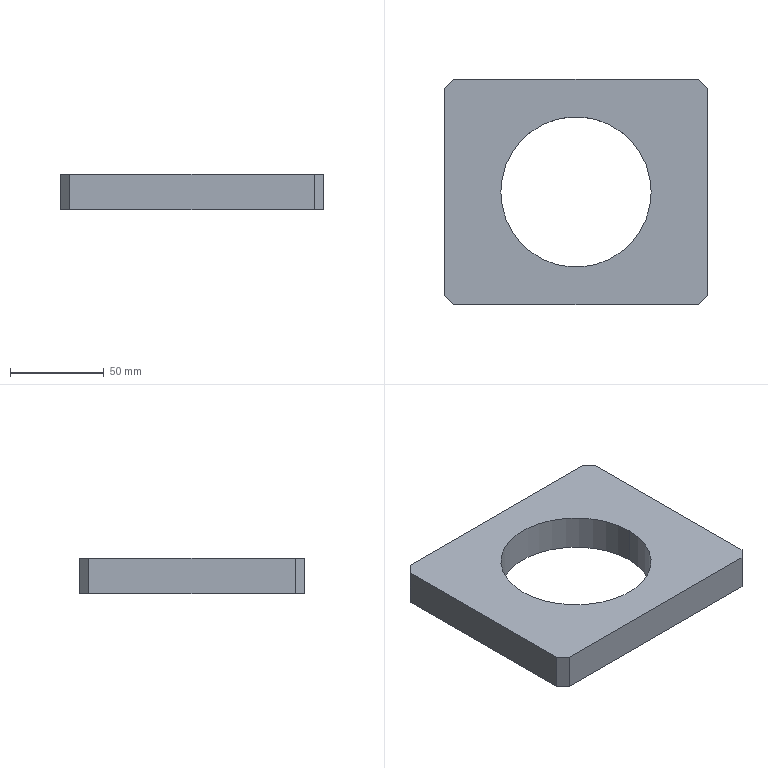Part | STEP file | Backup 2012-3-22-017 | 1 solid | 12 faces | box 140 x 120 x 19 mm | volume 222746 mm3 | plane 10 | cylinder 2 | commonest cylinder face diameters 80 x2
STEP:
#1=CARTESIAN_POINT('',(0.,0.,0.));
#2=DIRECTION('',(0.,0.,1.));
#3=DIRECTION('',(1.,0.,0.));
#4=AXIS2_PLACEMENT_3D('',#1,#2,#3);
#5=CARTESIAN_POINT('',(-40.,0.,19.));
#6=VERTEX_POINT('',#5);
#7=CARTESIAN_POINT('',(-40.,0.,0.));
#8=VERTEX_POINT('',#7);
#9=CARTESIAN_POINT('',(-40.,0.,19.));
#10=DIRECTION('',(0.,0.,-1.));
#11=VECTOR('',#10,1.);
#12=LINE('',#9,#11);
#13=CARTESIAN_POINT('',(0.,0.,19.));
#14=DIRECTION('',(0.,0.,-1.));
#15=DIRECTION('',(-1.,0.,0.));
#16=AXIS2_PLACEMENT_3D('',#13,#14,#15);
#17=CYLINDRICAL_SURFACE('',#16,40.);
#18=CARTESIAN_POINT('',(6.283,0.));
#19=DIRECTION('',(0.,1.));
#20=VECTOR('',#19,1.);
#21=LINE('',#18,#20);
#22=(GEOMETRIC_REPRESENTATION_CONTEXT(2)PARAMETRIC_REPRESENTATION_CONTEXT()REPRESENTATION_CONTEXT('',''));
#23=DEFINITIONAL_REPRESENTATION('',(#21),#22);
#24=PCURVE('',#17,#23);
#25=CARTESIAN_POINT('',(0.,0.,19.));
#26=DIRECTION('',(0.,0.,-1.));
#27=DIRECTION('',(-1.,0.,0.));
#28=AXIS2_PLACEMENT_3D('',#25,#26,#27);
#29=CYLINDRICAL_SURFACE('',#28,40.);
#30=CARTESIAN_POINT('',(0.,0.));
#31=DIRECTION('',(0.,1.));
#32=VECTOR('',#31,1.);
#33=LINE('',#30,#32);
#34=(GEOMETRIC_REPRESENTATION_CONTEXT(2)PARAMETRIC_REPRESENTATION_CONTEXT()REPRESENTATION_CONTEXT('',''));
#35=DEFINITIONAL_REPRESENTATION('',(#33),#34);
#36=PCURVE('',#29,#35);
#37=SURFACE_CURVE('',#12,(#24,#36),.PCURVE_S1.);
#38=EDGE_CURVE('',#6,#8,#37,.T.);
#39=ORIENTED_EDGE('',*,*,#38,.T.);
#40=CARTESIAN_POINT('',(40.,0.,0.));
#41=VERTEX_POINT('',#40);
#42=CARTESIAN_POINT('',(0.,0.,0.));
#43=DIRECTION('',(0.,0.,1.));
#44=DIRECTION('',(1.,0.,0.));
#45=AXIS2_PLACEMENT_3D('',#42,#43,#44);
#46=CIRCLE('',#45,40.);
#47=CARTESIAN_POINT('',(9.425,19.));
#48=DIRECTION('',(-1.,0.));
#49=VECTOR('',#48,1.);
#50=LINE('',#47,#49);
#51=(GEOMETRIC_REPRESENTATION_CONTEXT(2)PARAMETRIC_REPRESENTATION_CONTEXT()REPRESENTATION_CONTEXT('',''));
#52=DEFINITIONAL_REPRESENTATION('',(#50),#51);
#53=PCURVE('',#17,#52);
#54=CARTESIAN_POINT('',(70.,-60.,0.));
#55=DIRECTION('',(0.,0.,1.));
#56=DIRECTION('',(1.,0.,0.));
#57=AXIS2_PLACEMENT_3D('',#54,#55,#56);
#58=PLANE('',#57);
#59=CARTESIAN_POINT('',(-70.,60.));
#60=DIRECTION('',(1.,0.));
#61=AXIS2_PLACEMENT_2D('',#59,#60);
#62=CIRCLE('',#61,40.);
#63=(GEOMETRIC_REPRESENTATION_CONTEXT(2)PARAMETRIC_REPRESENTATION_CONTEXT()REPRESENTATION_CONTEXT('',''));
#64=DEFINITIONAL_REPRESENTATION('',(#62),#63);
#65=PCURVE('',#58,#64);
#66=SURFACE_CURVE('',#46,(#53,#65),.PCURVE_S1.);
#67=EDGE_CURVE('',#8,#41,#66,.T.);
#68=ORIENTED_EDGE('',*,*,#67,.T.);
#69=CARTESIAN_POINT('',(40.,0.,19.));
#70=VERTEX_POINT('',#69);
#71=CARTESIAN_POINT('',(40.,0.,19.));
#72=DIRECTION('',(0.,0.,-1.));
#73=VECTOR('',#72,1.);
#74=LINE('',#71,#73);
#75=CARTESIAN_POINT('',(3.142,0.));
#76=DIRECTION('',(0.,1.));
#77=VECTOR('',#76,1.);
#78=LINE('',#75,#77);
#79=(GEOMETRIC_REPRESENTATION_CONTEXT(2)PARAMETRIC_REPRESENTATION_CONTEXT()REPRESENTATION_CONTEXT('',''));
#80=DEFINITIONAL_REPRESENTATION('',(#78),#79);
#81=PCURVE('',#17,#80);
#82=CARTESIAN_POINT('',(3.142,0.));
#83=DIRECTION('',(0.,1.));
#84=VECTOR('',#83,1.);
#85=LINE('',#82,#84);
#86=(GEOMETRIC_REPRESENTATION_CONTEXT(2)PARAMETRIC_REPRESENTATION_CONTEXT()REPRESENTATION_CONTEXT('',''));
#87=DEFINITIONAL_REPRESENTATION('',(#85),#86);
#88=PCURVE('',#29,#87);
#89=SURFACE_CURVE('',#74,(#81,#88),.PCURVE_S1.);
#90=EDGE_CURVE('',#70,#41,#89,.T.);
#91=ORIENTED_EDGE('',*,*,#90,.F.);
#92=CARTESIAN_POINT('',(0.,0.,19.));
#93=DIRECTION('',(0.,0.,1.));
#94=DIRECTION('',(1.,0.,0.));
#95=AXIS2_PLACEMENT_3D('',#92,#93,#94);
#96=CIRCLE('',#95,40.);
#97=CARTESIAN_POINT('',(9.425,0.));
#98=DIRECTION('',(-1.,0.));
#99=VECTOR('',#98,1.);
#100=LINE('',#97,#99);
#101=(GEOMETRIC_REPRESENTATION_CONTEXT(2)PARAMETRIC_REPRESENTATION_CONTEXT()REPRESENTATION_CONTEXT('',''));
#102=DEFINITIONAL_REPRESENTATION('',(#100),#101);
#103=PCURVE('',#17,#102);
#104=CARTESIAN_POINT('',(70.,-60.,19.));
#105=DIRECTION('',(0.,0.,1.));
#106=DIRECTION('',(1.,0.,0.));
#107=AXIS2_PLACEMENT_3D('',#104,#105,#106);
#108=PLANE('',#107);
#109=CARTESIAN_POINT('',(-70.,60.));
#110=DIRECTION('',(1.,0.));
#111=AXIS2_PLACEMENT_2D('',#109,#110);
#112=CIRCLE('',#111,40.);
#113=(GEOMETRIC_REPRESENTATION_CONTEXT(2)PARAMETRIC_REPRESENTATION_CONTEXT()REPRESENTATION_CONTEXT('',''));
#114=DEFINITIONAL_REPRESENTATION('',(#112),#113);
#115=PCURVE('',#108,#114);
#116=SURFACE_CURVE('',#96,(#103,#115),.PCURVE_S1.);
#117=EDGE_CURVE('',#6,#70,#116,.T.);
#118=ORIENTED_EDGE('',*,*,#117,.F.);
#119=EDGE_LOOP('',(#39,#68,#91,#118));
#120=FACE_BOUND('',#119,.F.);
#121=ADVANCED_FACE('',(#120),#17,.F.);
#122=CARTESIAN_POINT('',(-70.,55.,19.));
#123=VERTEX_POINT('',#122);
#124=CARTESIAN_POINT('',(-70.,-55.,19.));
#125=VERTEX_POINT('',#124);
#126=CARTESIAN_POINT('',(-70.,60.,19.));
#127=DIRECTION('',(0.,-1.,0.));
#128=VECTOR('',#127,1.);
#129=LINE('',#126,#128);
#130=CARTESIAN_POINT('',(-140.,120.));
#131=DIRECTION('',(0.,-1.));
#132=VECTOR('',#131,1.);
#133=LINE('',#130,#132);
#134=(GEOMETRIC_REPRESENTATION_CONTEXT(2)PARAMETRIC_REPRESENTATION_CONTEXT()REPRESENTATION_CONTEXT('',''));
#135=DEFINITIONAL_REPRESENTATION('',(#133),#134);
#136=PCURVE('',#108,#135);
#137=CARTESIAN_POINT('',(-70.,60.,19.));
#138=DIRECTION('',(1.,0.,0.));
#139=DIRECTION('',(0.,0.,-1.));
#140=AXIS2_PLACEMENT_3D('',#137,#138,#139);
#141=PLANE('',#140);
#142=CARTESIAN_POINT('',(0.,0.));
#143=DIRECTION('',(0.,-1.));
#144=VECTOR('',#143,1.);
#145=LINE('',#142,#144);
#146=(GEOMETRIC_REPRESENTATION_CONTEXT(2)PARAMETRIC_REPRESENTATION_CONTEXT()REPRESENTATION_CONTEXT('',''));
#147=DEFINITIONAL_REPRESENTATION('',(#145),#146);
#148=PCURVE('',#141,#147);
#149=SURFACE_CURVE('',#129,(#136,#148),.PCURVE_S1.);
#150=EDGE_CURVE('',#123,#125,#149,.T.);
#151=ORIENTED_EDGE('',*,*,#150,.T.);
#152=CARTESIAN_POINT('',(-65.,-60.,19.));
#153=VERTEX_POINT('',#152);
#154=CARTESIAN_POINT('',(2.5,-127.5,19.));
#155=DIRECTION('',(0.7071,-0.7071,0.));
#156=VECTOR('',#155,1.);
#157=LINE('',#154,#156);
#158=CARTESIAN_POINT('',(-67.5,-67.5));
#159=DIRECTION('',(0.7071,-0.7071));
#160=VECTOR('',#159,1.);
#161=LINE('',#158,#160);
#162=(GEOMETRIC_REPRESENTATION_CONTEXT(2)PARAMETRIC_REPRESENTATION_CONTEXT()REPRESENTATION_CONTEXT('',''));
#163=DEFINITIONAL_REPRESENTATION('',(#161),#162);
#164=PCURVE('',#108,#163);
#165=CARTESIAN_POINT('',(-65.,-60.,19.));
#166=DIRECTION('',(0.7071,0.7071,0.));
#167=DIRECTION('',(-0.7071,0.7071,0.));
#168=AXIS2_PLACEMENT_3D('',#165,#166,#167);
#169=PLANE('',#168);
#170=CARTESIAN_POINT('',(-95.459,0.));
#171=DIRECTION('',(-1.,0.));
#172=VECTOR('',#171,1.);
#173=LINE('',#170,#172);
#174=(GEOMETRIC_REPRESENTATION_CONTEXT(2)PARAMETRIC_REPRESENTATION_CONTEXT()REPRESENTATION_CONTEXT('',''));
#175=DEFINITIONAL_REPRESENTATION('',(#173),#174);
#176=PCURVE('',#169,#175);
#177=SURFACE_CURVE('',#157,(#164,#176),.PCURVE_S1.);
#178=EDGE_CURVE('',#125,#153,#177,.T.);
#179=ORIENTED_EDGE('',*,*,#178,.T.);
#180=CARTESIAN_POINT('',(65.,-60.,19.));
#181=VERTEX_POINT('',#180);
#182=CARTESIAN_POINT('',(-70.,-60.,19.));
#183=DIRECTION('',(1.,0.,0.));
#184=VECTOR('',#183,1.);
#185=LINE('',#182,#184);
#186=CARTESIAN_POINT('',(-140.,0.));
#187=DIRECTION('',(1.,0.));
#188=VECTOR('',#187,1.);
#189=LINE('',#186,#188);
#190=(GEOMETRIC_REPRESENTATION_CONTEXT(2)PARAMETRIC_REPRESENTATION_CONTEXT()REPRESENTATION_CONTEXT('',''));
#191=DEFINITIONAL_REPRESENTATION('',(#189),#190);
#192=PCURVE('',#108,#191);
#193=CARTESIAN_POINT('',(-70.,-60.,19.));
#194=DIRECTION('',(0.,1.,0.));
#195=DIRECTION('',(0.,0.,1.));
#196=AXIS2_PLACEMENT_3D('',#193,#194,#195);
#197=PLANE('',#196);
#198=CARTESIAN_POINT('',(0.,0.));
#199=DIRECTION('',(0.,1.));
#200=VECTOR('',#199,1.);
#201=LINE('',#198,#200);
#202=(GEOMETRIC_REPRESENTATION_CONTEXT(2)PARAMETRIC_REPRESENTATION_CONTEXT()REPRESENTATION_CONTEXT('',''));
#203=DEFINITIONAL_REPRESENTATION('',(#201),#202);
#204=PCURVE('',#197,#203);
#205=SURFACE_CURVE('',#185,(#192,#204),.PCURVE_S1.);
#206=EDGE_CURVE('',#153,#181,#205,.T.);
#207=ORIENTED_EDGE('',*,*,#206,.T.);
#208=CARTESIAN_POINT('',(70.,-55.,19.));
#209=VERTEX_POINT('',#208);
#210=CARTESIAN_POINT('',(67.5,-57.5,19.));
#211=DIRECTION('',(0.7071,0.7071,0.));
#212=VECTOR('',#211,1.);
#213=LINE('',#210,#212);
#214=CARTESIAN_POINT('',(-2.5,2.5));
#215=DIRECTION('',(0.7071,0.7071));
#216=VECTOR('',#215,1.);
#217=LINE('',#214,#216);
#218=(GEOMETRIC_REPRESENTATION_CONTEXT(2)PARAMETRIC_REPRESENTATION_CONTEXT()REPRESENTATION_CONTEXT('',''));
#219=DEFINITIONAL_REPRESENTATION('',(#217),#218);
#220=PCURVE('',#108,#219);
#221=CARTESIAN_POINT('',(70.,-55.,19.));
#222=DIRECTION('',(-0.7071,0.7071,0.));
#223=DIRECTION('',(-0.7071,-0.7071,0.));
#224=AXIS2_PLACEMENT_3D('',#221,#222,#223);
#225=PLANE('',#224);
#226=CARTESIAN_POINT('',(3.536,0.));
#227=DIRECTION('',(-1.,0.));
#228=VECTOR('',#227,1.);
#229=LINE('',#226,#228);
#230=(GEOMETRIC_REPRESENTATION_CONTEXT(2)PARAMETRIC_REPRESENTATION_CONTEXT()REPRESENTATION_CONTEXT('',''));
#231=DEFINITIONAL_REPRESENTATION('',(#229),#230);
#232=PCURVE('',#225,#231);
#233=SURFACE_CURVE('',#213,(#220,#232),.PCURVE_S1.);
#234=EDGE_CURVE('',#181,#209,#233,.T.);
#235=ORIENTED_EDGE('',*,*,#234,.T.);
#236=CARTESIAN_POINT('',(70.,55.,19.));
#237=VERTEX_POINT('',#236);
#238=CARTESIAN_POINT('',(70.,60.,19.));
#239=DIRECTION('',(0.,1.,0.));
#240=VECTOR('',#239,1.);
#241=LINE('',#238,#240);
#242=CARTESIAN_POINT('',(0.,120.));
#243=DIRECTION('',(0.,1.));
#244=VECTOR('',#243,1.);
#245=LINE('',#242,#244);
#246=(GEOMETRIC_REPRESENTATION_CONTEXT(2)PARAMETRIC_REPRESENTATION_CONTEXT()REPRESENTATION_CONTEXT('',''));
#247=DEFINITIONAL_REPRESENTATION('',(#245),#246);
#248=PCURVE('',#108,#247);
#249=CARTESIAN_POINT('',(70.,60.,19.));
#250=DIRECTION('',(-1.,0.,0.));
#251=DIRECTION('',(0.,0.,1.));
#252=AXIS2_PLACEMENT_3D('',#249,#250,#251);
#253=PLANE('',#252);
#254=CARTESIAN_POINT('',(0.,0.));
#255=DIRECTION('',(0.,1.));
#256=VECTOR('',#255,1.);
#257=LINE('',#254,#256);
#258=(GEOMETRIC_REPRESENTATION_CONTEXT(2)PARAMETRIC_REPRESENTATION_CONTEXT()REPRESENTATION_CONTEXT('',''));
#259=DEFINITIONAL_REPRESENTATION('',(#257),#258);
#260=PCURVE('',#253,#259);
#261=SURFACE_CURVE('',#241,(#248,#260),.PCURVE_S1.);
#262=EDGE_CURVE('',#209,#237,#261,.T.);
#263=ORIENTED_EDGE('',*,*,#262,.T.);
#264=CARTESIAN_POINT('',(65.,60.,19.));
#265=VERTEX_POINT('',#264);
#266=CARTESIAN_POINT('',(127.5,-2.5,19.));
#267=DIRECTION('',(-0.7071,0.7071,0.));
#268=VECTOR('',#267,1.);
#269=LINE('',#266,#268);
#270=CARTESIAN_POINT('',(57.5,57.5));
#271=DIRECTION('',(-0.7071,0.7071));
#272=VECTOR('',#271,1.);
#273=LINE('',#270,#272);
#274=(GEOMETRIC_REPRESENTATION_CONTEXT(2)PARAMETRIC_REPRESENTATION_CONTEXT()REPRESENTATION_CONTEXT('',''));
#275=DEFINITIONAL_REPRESENTATION('',(#273),#274);
#276=PCURVE('',#108,#275);
#277=CARTESIAN_POINT('',(65.,60.,19.));
#278=DIRECTION('',(-0.7071,-0.7071,0.));
#279=DIRECTION('',(0.7071,-0.7071,0.));
#280=AXIS2_PLACEMENT_3D('',#277,#278,#279);
#281=PLANE('',#280);
#282=CARTESIAN_POINT('',(88.388,0.));
#283=DIRECTION('',(-1.,0.));
#284=VECTOR('',#283,1.);
#285=LINE('',#282,#284);
#286=(GEOMETRIC_REPRESENTATION_CONTEXT(2)PARAMETRIC_REPRESENTATION_CONTEXT()REPRESENTATION_CONTEXT('',''));
#287=DEFINITIONAL_REPRESENTATION('',(#285),#286);
#288=PCURVE('',#281,#287);
#289=SURFACE_CURVE('',#269,(#276,#288),.PCURVE_S1.);
#290=EDGE_CURVE('',#237,#265,#289,.T.);
#291=ORIENTED_EDGE('',*,*,#290,.T.);
#292=CARTESIAN_POINT('',(-65.,60.,19.));
#293=VERTEX_POINT('',#292);
#294=CARTESIAN_POINT('',(-70.,60.,19.));
#295=DIRECTION('',(-1.,0.,0.));
#296=VECTOR('',#295,1.);
#297=LINE('',#294,#296);
#298=CARTESIAN_POINT('',(-140.,120.));
#299=DIRECTION('',(-1.,0.));
#300=VECTOR('',#299,1.);
#301=LINE('',#298,#300);
#302=(GEOMETRIC_REPRESENTATION_CONTEXT(2)PARAMETRIC_REPRESENTATION_CONTEXT()REPRESENTATION_CONTEXT('',''));
#303=DEFINITIONAL_REPRESENTATION('',(#301),#302);
#304=PCURVE('',#108,#303);
#305=CARTESIAN_POINT('',(-70.,60.,19.));
#306=DIRECTION('',(0.,-1.,0.));
#307=DIRECTION('',(0.,0.,-1.));
#308=AXIS2_PLACEMENT_3D('',#305,#306,#307);
#309=PLANE('',#308);
#310=CARTESIAN_POINT('',(0.,0.));
#311=DIRECTION('',(0.,-1.));
#312=VECTOR('',#311,1.);
#313=LINE('',#310,#312);
#314=(GEOMETRIC_REPRESENTATION_CONTEXT(2)PARAMETRIC_REPRESENTATION_CONTEXT()REPRESENTATION_CONTEXT('',''));
#315=DEFINITIONAL_REPRESENTATION('',(#313),#314);
#316=PCURVE('',#309,#315);
#317=SURFACE_CURVE('',#297,(#304,#316),.PCURVE_S1.);
#318=EDGE_CURVE('',#265,#293,#317,.T.);
#319=ORIENTED_EDGE('',*,*,#318,.T.);
#320=CARTESIAN_POINT('',(-57.5,67.5,19.));
#321=DIRECTION('',(-0.7071,-0.7071,0.));
#322=VECTOR('',#321,1.);
#323=LINE('',#320,#322);
#324=CARTESIAN_POINT('',(-127.5,127.5));
#325=DIRECTION('',(-0.7071,-0.7071));
#326=VECTOR('',#325,1.);
#327=LINE('',#324,#326);
#328=(GEOMETRIC_REPRESENTATION_CONTEXT(2)PARAMETRIC_REPRESENTATION_CONTEXT()REPRESENTATION_CONTEXT('',''));
#329=DEFINITIONAL_REPRESENTATION('',(#327),#328);
#330=PCURVE('',#108,#329);
#331=CARTESIAN_POINT('',(-70.,55.,19.));
#332=DIRECTION('',(0.7071,-0.7071,0.));
#333=DIRECTION('',(0.7071,0.7071,0.));
#334=AXIS2_PLACEMENT_3D('',#331,#332,#333);
#335=PLANE('',#334);
#336=CARTESIAN_POINT('',(17.678,0.));
#337=DIRECTION('',(-1.,0.));
#338=VECTOR('',#337,1.);
#339=LINE('',#336,#338);
#340=(GEOMETRIC_REPRESENTATION_CONTEXT(2)PARAMETRIC_REPRESENTATION_CONTEXT()REPRESENTATION_CONTEXT('',''));
#341=DEFINITIONAL_REPRESENTATION('',(#339),#340);
#342=PCURVE('',#335,#341);
#343=SURFACE_CURVE('',#323,(#330,#342),.PCURVE_S1.);
#344=EDGE_CURVE('',#293,#123,#343,.T.);
#345=ORIENTED_EDGE('',*,*,#344,.T.);
#346=EDGE_LOOP('',(#151,#179,#207,#235,#263,#291,#319,#345));
#347=FACE_BOUND('',#346,.T.);
#348=ORIENTED_EDGE('',*,*,#117,.F.);
#349=CARTESIAN_POINT('',(0.,0.,19.));
#350=DIRECTION('',(0.,0.,1.));
#351=DIRECTION('',(1.,0.,0.));
#352=AXIS2_PLACEMENT_3D('',#349,#350,#351);
#353=CIRCLE('',#352,40.);
#354=CARTESIAN_POINT('',(-70.,60.));
#355=DIRECTION('',(1.,0.));
#356=AXIS2_PLACEMENT_2D('',#354,#355);
#357=CIRCLE('',#356,40.);
#358=(GEOMETRIC_REPRESENTATION_CONTEXT(2)PARAMETRIC_REPRESENTATION_CONTEXT()REPRESENTATION_CONTEXT('',''));
#359=DEFINITIONAL_REPRESENTATION('',(#357),#358);
#360=PCURVE('',#108,#359);
#361=CARTESIAN_POINT('',(3.142,0.));
#362=DIRECTION('',(-1.,0.));
#363=VECTOR('',#362,1.);
#364=LINE('',#361,#363);
#365=(GEOMETRIC_REPRESENTATION_CONTEXT(2)PARAMETRIC_REPRESENTATION_CONTEXT()REPRESENTATION_CONTEXT('',''));
#366=DEFINITIONAL_REPRESENTATION('',(#364),#365);
#367=PCURVE('',#29,#366);
#368=SURFACE_CURVE('',#353,(#360,#367),.PCURVE_S1.);
#369=EDGE_CURVE('',#70,#6,#368,.T.);
#370=ORIENTED_EDGE('',*,*,#369,.F.);
#371=EDGE_LOOP('',(#348,#370));
#372=FACE_BOUND('',#371,.T.);
#373=ADVANCED_FACE('',(#347,#372),#108,.T.);
#374=CARTESIAN_POINT('',(-65.,-60.,0.));
#375=VERTEX_POINT('',#374);
#376=CARTESIAN_POINT('',(65.,-60.,0.));
#377=VERTEX_POINT('',#376);
#378=CARTESIAN_POINT('',(-70.,-60.,0.));
#379=DIRECTION('',(1.,0.,0.));
#380=VECTOR('',#379,1.);
#381=LINE('',#378,#380);
#382=CARTESIAN_POINT('',(-140.,0.));
#383=DIRECTION('',(1.,0.));
#384=VECTOR('',#383,1.);
#385=LINE('',#382,#384);
#386=(GEOMETRIC_REPRESENTATION_CONTEXT(2)PARAMETRIC_REPRESENTATION_CONTEXT()REPRESENTATION_CONTEXT('',''));
#387=DEFINITIONAL_REPRESENTATION('',(#385),#386);
#388=PCURVE('',#58,#387);
#389=CARTESIAN_POINT('',(-19.,0.));
#390=DIRECTION('',(0.,1.));
#391=VECTOR('',#390,1.);
#392=LINE('',#389,#391);
#393=(GEOMETRIC_REPRESENTATION_CONTEXT(2)PARAMETRIC_REPRESENTATION_CONTEXT()REPRESENTATION_CONTEXT('',''));
#394=DEFINITIONAL_REPRESENTATION('',(#392),#393);
#395=PCURVE('',#197,#394);
#396=SURFACE_CURVE('',#381,(#388,#395),.PCURVE_S1.);
#397=EDGE_CURVE('',#375,#377,#396,.T.);
#398=ORIENTED_EDGE('',*,*,#397,.F.);
#399=CARTESIAN_POINT('',(-70.,-55.,0.));
#400=VERTEX_POINT('',#399);
#401=CARTESIAN_POINT('',(-65.,-60.,0.));
#402=DIRECTION('',(-0.7071,0.7071,0.));
#403=VECTOR('',#402,1.);
#404=LINE('',#401,#403);
#405=CARTESIAN_POINT('',(-135.,0.));
#406=DIRECTION('',(-0.7071,0.7071));
#407=VECTOR('',#406,1.);
#408=LINE('',#405,#407);
#409=(GEOMETRIC_REPRESENTATION_CONTEXT(2)PARAMETRIC_REPRESENTATION_CONTEXT()REPRESENTATION_CONTEXT('',''));
#410=DEFINITIONAL_REPRESENTATION('',(#408),#409);
#411=PCURVE('',#58,#410);
#412=CARTESIAN_POINT('',(0.,-19.));
#413=DIRECTION('',(1.,0.));
#414=VECTOR('',#413,1.);
#415=LINE('',#412,#414);
#416=(GEOMETRIC_REPRESENTATION_CONTEXT(2)PARAMETRIC_REPRESENTATION_CONTEXT()REPRESENTATION_CONTEXT('',''));
#417=DEFINITIONAL_REPRESENTATION('',(#415),#416);
#418=PCURVE('',#169,#417);
#419=SURFACE_CURVE('',#404,(#411,#418),.PCURVE_S1.);
#420=EDGE_CURVE('',#375,#400,#419,.T.);
#421=ORIENTED_EDGE('',*,*,#420,.T.);
#422=CARTESIAN_POINT('',(-70.,55.,0.));
#423=VERTEX_POINT('',#422);
#424=CARTESIAN_POINT('',(-70.,60.,0.));
#425=DIRECTION('',(0.,-1.,0.));
#426=VECTOR('',#425,1.);
#427=LINE('',#424,#426);
#428=CARTESIAN_POINT('',(-140.,120.));
#429=DIRECTION('',(0.,-1.));
#430=VECTOR('',#429,1.);
#431=LINE('',#428,#430);
#432=(GEOMETRIC_REPRESENTATION_CONTEXT(2)PARAMETRIC_REPRESENTATION_CONTEXT()REPRESENTATION_CONTEXT('',''));
#433=DEFINITIONAL_REPRESENTATION('',(#431),#432);
#434=PCURVE('',#58,#433);
#435=CARTESIAN_POINT('',(19.,0.));
#436=DIRECTION('',(0.,-1.));
#437=VECTOR('',#436,1.);
#438=LINE('',#435,#437);
#439=(GEOMETRIC_REPRESENTATION_CONTEXT(2)PARAMETRIC_REPRESENTATION_CONTEXT()REPRESENTATION_CONTEXT('',''));
#440=DEFINITIONAL_REPRESENTATION('',(#438),#439);
#441=PCURVE('',#141,#440);
#442=SURFACE_CURVE('',#427,(#434,#441),.PCURVE_S1.);
#443=EDGE_CURVE('',#423,#400,#442,.T.);
#444=ORIENTED_EDGE('',*,*,#443,.F.);
#445=CARTESIAN_POINT('',(-65.,60.,0.));
#446=VERTEX_POINT('',#445);
#447=CARTESIAN_POINT('',(-70.,55.,0.));
#448=DIRECTION('',(0.7071,0.7071,0.));
#449=VECTOR('',#448,1.);
#450=LINE('',#447,#449);
#451=CARTESIAN_POINT('',(-140.,115.));
#452=DIRECTION('',(0.7071,0.7071));
#453=VECTOR('',#452,1.);
#454=LINE('',#451,#453);
#455=(GEOMETRIC_REPRESENTATION_CONTEXT(2)PARAMETRIC_REPRESENTATION_CONTEXT()REPRESENTATION_CONTEXT('',''));
#456=DEFINITIONAL_REPRESENTATION('',(#454),#455);
#457=PCURVE('',#58,#456);
#458=CARTESIAN_POINT('',(0.,-19.));
#459=DIRECTION('',(1.,0.));
#460=VECTOR('',#459,1.);
#461=LINE('',#458,#460);
#462=(GEOMETRIC_REPRESENTATION_CONTEXT(2)PARAMETRIC_REPRESENTATION_CONTEXT()REPRESENTATION_CONTEXT('',''));
#463=DEFINITIONAL_REPRESENTATION('',(#461),#462);
#464=PCURVE('',#335,#463);
#465=SURFACE_CURVE('',#450,(#457,#464),.PCURVE_S1.);
#466=EDGE_CURVE('',#423,#446,#465,.T.);
#467=ORIENTED_EDGE('',*,*,#466,.T.);
#468=CARTESIAN_POINT('',(65.,60.,0.));
#469=VERTEX_POINT('',#468);
#470=CARTESIAN_POINT('',(-70.,60.,0.));
#471=DIRECTION('',(-1.,0.,0.));
#472=VECTOR('',#471,1.);
#473=LINE('',#470,#472);
#474=CARTESIAN_POINT('',(-140.,120.));
#475=DIRECTION('',(-1.,0.));
#476=VECTOR('',#475,1.);
#477=LINE('',#474,#476);
#478=(GEOMETRIC_REPRESENTATION_CONTEXT(2)PARAMETRIC_REPRESENTATION_CONTEXT()REPRESENTATION_CONTEXT('',''));
#479=DEFINITIONAL_REPRESENTATION('',(#477),#478);
#480=PCURVE('',#58,#479);
#481=CARTESIAN_POINT('',(19.,0.));
#482=DIRECTION('',(0.,-1.));
#483=VECTOR('',#482,1.);
#484=LINE('',#481,#483);
#485=(GEOMETRIC_REPRESENTATION_CONTEXT(2)PARAMETRIC_REPRESENTATION_CONTEXT()REPRESENTATION_CONTEXT('',''));
#486=DEFINITIONAL_REPRESENTATION('',(#484),#485);
#487=PCURVE('',#309,#486);
#488=SURFACE_CURVE('',#473,(#480,#487),.PCURVE_S1.);
#489=EDGE_CURVE('',#469,#446,#488,.T.);
#490=ORIENTED_EDGE('',*,*,#489,.F.);
#491=CARTESIAN_POINT('',(70.,55.,0.));
#492=VERTEX_POINT('',#491);
#493=CARTESIAN_POINT('',(65.,60.,0.));
#494=DIRECTION('',(0.7071,-0.7071,0.));
#495=VECTOR('',#494,1.);
#496=LINE('',#493,#495);
#497=CARTESIAN_POINT('',(-5.,120.));
#498=DIRECTION('',(0.7071,-0.7071));
#499=VECTOR('',#498,1.);
#500=LINE('',#497,#499);
#501=(GEOMETRIC_REPRESENTATION_CONTEXT(2)PARAMETRIC_REPRESENTATION_CONTEXT()REPRESENTATION_CONTEXT('',''));
#502=DEFINITIONAL_REPRESENTATION('',(#500),#501);
#503=PCURVE('',#58,#502);
#504=CARTESIAN_POINT('',(0.,-19.));
#505=DIRECTION('',(1.,0.));
#506=VECTOR('',#505,1.);
#507=LINE('',#504,#506);
#508=(GEOMETRIC_REPRESENTATION_CONTEXT(2)PARAMETRIC_REPRESENTATION_CONTEXT()REPRESENTATION_CONTEXT('',''));
#509=DEFINITIONAL_REPRESENTATION('',(#507),#508);
#510=PCURVE('',#281,#509);
#511=SURFACE_CURVE('',#496,(#503,#510),.PCURVE_S1.);
#512=EDGE_CURVE('',#469,#492,#511,.T.);
#513=ORIENTED_EDGE('',*,*,#512,.T.);
#514=CARTESIAN_POINT('',(70.,-55.,0.));
#515=VERTEX_POINT('',#514);
#516=CARTESIAN_POINT('',(70.,60.,0.));
#517=DIRECTION('',(0.,1.,0.));
#518=VECTOR('',#517,1.);
#519=LINE('',#516,#518);
#520=CARTESIAN_POINT('',(0.,120.));
#521=DIRECTION('',(0.,1.));
#522=VECTOR('',#521,1.);
#523=LINE('',#520,#522);
#524=(GEOMETRIC_REPRESENTATION_CONTEXT(2)PARAMETRIC_REPRESENTATION_CONTEXT()REPRESENTATION_CONTEXT('',''));
#525=DEFINITIONAL_REPRESENTATION('',(#523),#524);
#526=PCURVE('',#58,#525);
#527=CARTESIAN_POINT('',(-19.,0.));
#528=DIRECTION('',(0.,1.));
#529=VECTOR('',#528,1.);
#530=LINE('',#527,#529);
#531=(GEOMETRIC_REPRESENTATION_CONTEXT(2)PARAMETRIC_REPRESENTATION_CONTEXT()REPRESENTATION_CONTEXT('',''));
#532=DEFINITIONAL_REPRESENTATION('',(#530),#531);
#533=PCURVE('',#253,#532);
#534=SURFACE_CURVE('',#519,(#526,#533),.PCURVE_S1.);
#535=EDGE_CURVE('',#515,#492,#534,.T.);
#536=ORIENTED_EDGE('',*,*,#535,.F.);
#537=CARTESIAN_POINT('',(70.,-55.,0.));
#538=DIRECTION('',(-0.7071,-0.7071,0.));
#539=VECTOR('',#538,1.);
#540=LINE('',#537,#539);
#541=CARTESIAN_POINT('',(0.,5.));
#542=DIRECTION('',(-0.7071,-0.7071));
#543=VECTOR('',#542,1.);
#544=LINE('',#541,#543);
#545=(GEOMETRIC_REPRESENTATION_CONTEXT(2)PARAMETRIC_REPRESENTATION_CONTEXT()REPRESENTATION_CONTEXT('',''));
#546=DEFINITIONAL_REPRESENTATION('',(#544),#545);
#547=PCURVE('',#58,#546);
#548=CARTESIAN_POINT('',(0.,-19.));
#549=DIRECTION('',(1.,0.));
#550=VECTOR('',#549,1.);
#551=LINE('',#548,#550);
#552=(GEOMETRIC_REPRESENTATION_CONTEXT(2)PARAMETRIC_REPRESENTATION_CONTEXT()REPRESENTATION_CONTEXT('',''));
#553=DEFINITIONAL_REPRESENTATION('',(#551),#552);
#554=PCURVE('',#225,#553);
#555=SURFACE_CURVE('',#540,(#547,#554),.PCURVE_S1.);
#556=EDGE_CURVE('',#515,#377,#555,.T.);
#557=ORIENTED_EDGE('',*,*,#556,.T.);
#558=EDGE_LOOP('',(#398,#421,#444,#467,#490,#513,#536,#557));
#559=FACE_BOUND('',#558,.T.);
#560=ORIENTED_EDGE('',*,*,#67,.T.);
#561=CARTESIAN_POINT('',(0.,0.,0.));
#562=DIRECTION('',(0.,0.,1.));
#563=DIRECTION('',(1.,0.,0.));
#564=AXIS2_PLACEMENT_3D('',#561,#562,#563);
#565=CIRCLE('',#564,40.);
#566=CARTESIAN_POINT('',(-70.,60.));
#567=DIRECTION('',(1.,0.));
#568=AXIS2_PLACEMENT_2D('',#566,#567);
#569=CIRCLE('',#568,40.);
#570=(GEOMETRIC_REPRESENTATION_CONTEXT(2)PARAMETRIC_REPRESENTATION_CONTEXT()REPRESENTATION_CONTEXT('',''));
#571=DEFINITIONAL_REPRESENTATION('',(#569),#570);
#572=PCURVE('',#58,#571);
#573=CARTESIAN_POINT('',(3.142,19.));
#574=DIRECTION('',(-1.,0.));
#575=VECTOR('',#574,1.);
#576=LINE('',#573,#575);
#577=(GEOMETRIC_REPRESENTATION_CONTEXT(2)PARAMETRIC_REPRESENTATION_CONTEXT()REPRESENTATION_CONTEXT('',''));
#578=DEFINITIONAL_REPRESENTATION('',(#576),#577);
#579=PCURVE('',#29,#578);
#580=SURFACE_CURVE('',#565,(#572,#579),.PCURVE_S1.);
#581=EDGE_CURVE('',#41,#8,#580,.T.);
#582=ORIENTED_EDGE('',*,*,#581,.T.);
#583=EDGE_LOOP('',(#560,#582));
#584=FACE_BOUND('',#583,.T.);
#585=ADVANCED_FACE('',(#559,#584),#58,.F.);
#586=ORIENTED_EDGE('',*,*,#262,.F.);
#587=CARTESIAN_POINT('',(70.,-55.,19.));
#588=DIRECTION('',(0.,0.,-1.));
#589=VECTOR('',#588,1.);
#590=LINE('',#587,#589);
#591=CARTESIAN_POINT('',(0.,-115.));
#592=DIRECTION('',(-1.,0.));
#593=VECTOR('',#592,1.);
#594=LINE('',#591,#593);
#595=(GEOMETRIC_REPRESENTATION_CONTEXT(2)PARAMETRIC_REPRESENTATION_CONTEXT()REPRESENTATION_CONTEXT('',''));
#596=DEFINITIONAL_REPRESENTATION('',(#594),#595);
#597=PCURVE('',#253,#596);
#598=CARTESIAN_POINT('',(0.,0.));
#599=DIRECTION('',(0.,-1.));
#600=VECTOR('',#599,1.);
#601=LINE('',#598,#600);
#602=(GEOMETRIC_REPRESENTATION_CONTEXT(2)PARAMETRIC_REPRESENTATION_CONTEXT()REPRESENTATION_CONTEXT('',''));
#603=DEFINITIONAL_REPRESENTATION('',(#601),#602);
#604=PCURVE('',#225,#603);
#605=SURFACE_CURVE('',#590,(#597,#604),.PCURVE_S1.);
#606=EDGE_CURVE('',#209,#515,#605,.T.);
#607=ORIENTED_EDGE('',*,*,#606,.T.);
#608=ORIENTED_EDGE('',*,*,#535,.T.);
#609=CARTESIAN_POINT('',(70.,55.,19.));
#610=DIRECTION('',(0.,0.,1.));
#611=VECTOR('',#610,1.);
#612=LINE('',#609,#611);
#613=CARTESIAN_POINT('',(0.,-5.));
#614=DIRECTION('',(1.,0.));
#615=VECTOR('',#614,1.);
#616=LINE('',#613,#615);
#617=(GEOMETRIC_REPRESENTATION_CONTEXT(2)PARAMETRIC_REPRESENTATION_CONTEXT()REPRESENTATION_CONTEXT('',''));
#618=DEFINITIONAL_REPRESENTATION('',(#616),#617);
#619=PCURVE('',#253,#618);
#620=CARTESIAN_POINT('',(7.071,0.));
#621=DIRECTION('',(0.,1.));
#622=VECTOR('',#621,1.);
#623=LINE('',#620,#622);
#624=(GEOMETRIC_REPRESENTATION_CONTEXT(2)PARAMETRIC_REPRESENTATION_CONTEXT()REPRESENTATION_CONTEXT('',''));
#625=DEFINITIONAL_REPRESENTATION('',(#623),#624);
#626=PCURVE('',#281,#625);
#627=SURFACE_CURVE('',#612,(#619,#626),.PCURVE_S1.);
#628=EDGE_CURVE('',#492,#237,#627,.T.);
#629=ORIENTED_EDGE('',*,*,#628,.T.);
#630=EDGE_LOOP('',(#586,#607,#608,#629));
#631=FACE_BOUND('',#630,.T.);
#632=ADVANCED_FACE('',(#631),#253,.F.);
#633=ORIENTED_EDGE('',*,*,#489,.T.);
#634=CARTESIAN_POINT('',(-65.,60.,19.));
#635=DIRECTION('',(0.,0.,1.));
#636=VECTOR('',#635,1.);
#637=LINE('',#634,#636);
#638=CARTESIAN_POINT('',(0.,5.));
#639=DIRECTION('',(-1.,0.));
#640=VECTOR('',#639,1.);
#641=LINE('',#638,#640);
#642=(GEOMETRIC_REPRESENTATION_CONTEXT(2)PARAMETRIC_REPRESENTATION_CONTEXT()REPRESENTATION_CONTEXT('',''));
#643=DEFINITIONAL_REPRESENTATION('',(#641),#642);
#644=PCURVE('',#309,#643);
#645=CARTESIAN_POINT('',(7.071,0.));
#646=DIRECTION('',(0.,1.));
#647=VECTOR('',#646,1.);
#648=LINE('',#645,#647);
#649=(GEOMETRIC_REPRESENTATION_CONTEXT(2)PARAMETRIC_REPRESENTATION_CONTEXT()REPRESENTATION_CONTEXT('',''));
#650=DEFINITIONAL_REPRESENTATION('',(#648),#649);
#651=PCURVE('',#335,#650);
#652=SURFACE_CURVE('',#637,(#644,#651),.PCURVE_S1.);
#653=EDGE_CURVE('',#446,#293,#652,.T.);
#654=ORIENTED_EDGE('',*,*,#653,.T.);
#655=ORIENTED_EDGE('',*,*,#318,.F.);
#656=CARTESIAN_POINT('',(65.,60.,19.));
#657=DIRECTION('',(0.,0.,-1.));
#658=VECTOR('',#657,1.);
#659=LINE('',#656,#658);
#660=CARTESIAN_POINT('',(0.,135.));
#661=DIRECTION('',(1.,0.));
#662=VECTOR('',#661,1.);
#663=LINE('',#660,#662);
#664=(GEOMETRIC_REPRESENTATION_CONTEXT(2)PARAMETRIC_REPRESENTATION_CONTEXT()REPRESENTATION_CONTEXT('',''));
#665=DEFINITIONAL_REPRESENTATION('',(#663),#664);
#666=PCURVE('',#309,#665);
#667=CARTESIAN_POINT('',(0.,0.));
#668=DIRECTION('',(0.,-1.));
#669=VECTOR('',#668,1.);
#670=LINE('',#667,#669);
#671=(GEOMETRIC_REPRESENTATION_CONTEXT(2)PARAMETRIC_REPRESENTATION_CONTEXT()REPRESENTATION_CONTEXT('',''));
#672=DEFINITIONAL_REPRESENTATION('',(#670),#671);
#673=PCURVE('',#281,#672);
#674=SURFACE_CURVE('',#659,(#666,#673),.PCURVE_S1.);
#675=EDGE_CURVE('',#265,#469,#674,.T.);
#676=ORIENTED_EDGE('',*,*,#675,.T.);
#677=EDGE_LOOP('',(#633,#654,#655,#676));
#678=FACE_BOUND('',#677,.T.);
#679=ADVANCED_FACE('',(#678),#309,.F.);
#680=ORIENTED_EDGE('',*,*,#443,.T.);
#681=CARTESIAN_POINT('',(-70.,-55.,19.));
#682=DIRECTION('',(0.,0.,1.));
#683=VECTOR('',#682,1.);
#684=LINE('',#681,#683);
#685=CARTESIAN_POINT('',(0.,-115.));
#686=DIRECTION('',(-1.,0.));
#687=VECTOR('',#686,1.);
#688=LINE('',#685,#687);
#689=(GEOMETRIC_REPRESENTATION_CONTEXT(2)PARAMETRIC_REPRESENTATION_CONTEXT()REPRESENTATION_CONTEXT('',''));
#690=DEFINITIONAL_REPRESENTATION('',(#688),#689);
#691=PCURVE('',#141,#690);
#692=CARTESIAN_POINT('',(7.071,0.));
#693=DIRECTION('',(0.,1.));
#694=VECTOR('',#693,1.);
#695=LINE('',#692,#694);
#696=(GEOMETRIC_REPRESENTATION_CONTEXT(2)PARAMETRIC_REPRESENTATION_CONTEXT()REPRESENTATION_CONTEXT('',''));
#697=DEFINITIONAL_REPRESENTATION('',(#695),#696);
#698=PCURVE('',#169,#697);
#699=SURFACE_CURVE('',#684,(#691,#698),.PCURVE_S1.);
#700=EDGE_CURVE('',#400,#125,#699,.T.);
#701=ORIENTED_EDGE('',*,*,#700,.T.);
#702=ORIENTED_EDGE('',*,*,#150,.F.);
#703=CARTESIAN_POINT('',(-70.,55.,19.));
#704=DIRECTION('',(0.,0.,-1.));
#705=VECTOR('',#704,1.);
#706=LINE('',#703,#705);
#707=CARTESIAN_POINT('',(0.,-5.));
#708=DIRECTION('',(1.,0.));
#709=VECTOR('',#708,1.);
#710=LINE('',#707,#709);
#711=(GEOMETRIC_REPRESENTATION_CONTEXT(2)PARAMETRIC_REPRESENTATION_CONTEXT()REPRESENTATION_CONTEXT('',''));
#712=DEFINITIONAL_REPRESENTATION('',(#710),#711);
#713=PCURVE('',#141,#712);
#714=CARTESIAN_POINT('',(0.,0.));
#715=DIRECTION('',(0.,-1.));
#716=VECTOR('',#715,1.);
#717=LINE('',#714,#716);
#718=(GEOMETRIC_REPRESENTATION_CONTEXT(2)PARAMETRIC_REPRESENTATION_CONTEXT()REPRESENTATION_CONTEXT('',''));
#719=DEFINITIONAL_REPRESENTATION('',(#717),#718);
#720=PCURVE('',#335,#719);
#721=SURFACE_CURVE('',#706,(#713,#720),.PCURVE_S1.);
#722=EDGE_CURVE('',#123,#423,#721,.T.);
#723=ORIENTED_EDGE('',*,*,#722,.T.);
#724=EDGE_LOOP('',(#680,#701,#702,#723));
#725=FACE_BOUND('',#724,.T.);
#726=ADVANCED_FACE('',(#725),#141,.F.);
#727=ORIENTED_EDGE('',*,*,#206,.F.);
#728=CARTESIAN_POINT('',(-65.,-60.,19.));
#729=DIRECTION('',(0.,0.,-1.));
#730=VECTOR('',#729,1.);
#731=LINE('',#728,#730);
#732=CARTESIAN_POINT('',(0.,5.));
#733=DIRECTION('',(-1.,0.));
#734=VECTOR('',#733,1.);
#735=LINE('',#732,#734);
#736=(GEOMETRIC_REPRESENTATION_CONTEXT(2)PARAMETRIC_REPRESENTATION_CONTEXT()REPRESENTATION_CONTEXT('',''));
#737=DEFINITIONAL_REPRESENTATION('',(#735),#736);
#738=PCURVE('',#197,#737);
#739=CARTESIAN_POINT('',(0.,0.));
#740=DIRECTION('',(0.,-1.));
#741=VECTOR('',#740,1.);
#742=LINE('',#739,#741);
#743=(GEOMETRIC_REPRESENTATION_CONTEXT(2)PARAMETRIC_REPRESENTATION_CONTEXT()REPRESENTATION_CONTEXT('',''));
#744=DEFINITIONAL_REPRESENTATION('',(#742),#743);
#745=PCURVE('',#169,#744);
#746=SURFACE_CURVE('',#731,(#738,#745),.PCURVE_S1.);
#747=EDGE_CURVE('',#153,#375,#746,.T.);
#748=ORIENTED_EDGE('',*,*,#747,.T.);
#749=ORIENTED_EDGE('',*,*,#397,.T.);
#750=CARTESIAN_POINT('',(65.,-60.,19.));
#751=DIRECTION('',(0.,0.,1.));
#752=VECTOR('',#751,1.);
#753=LINE('',#750,#752);
#754=CARTESIAN_POINT('',(0.,135.));
#755=DIRECTION('',(1.,0.));
#756=VECTOR('',#755,1.);
#757=LINE('',#754,#756);
#758=(GEOMETRIC_REPRESENTATION_CONTEXT(2)PARAMETRIC_REPRESENTATION_CONTEXT()REPRESENTATION_CONTEXT('',''));
#759=DEFINITIONAL_REPRESENTATION('',(#757),#758);
#760=PCURVE('',#197,#759);
#761=CARTESIAN_POINT('',(7.071,0.));
#762=DIRECTION('',(0.,1.));
#763=VECTOR('',#762,1.);
#764=LINE('',#761,#763);
#765=(GEOMETRIC_REPRESENTATION_CONTEXT(2)PARAMETRIC_REPRESENTATION_CONTEXT()REPRESENTATION_CONTEXT('',''));
#766=DEFINITIONAL_REPRESENTATION('',(#764),#765);
#767=PCURVE('',#225,#766);
#768=SURFACE_CURVE('',#753,(#760,#767),.PCURVE_S1.);
#769=EDGE_CURVE('',#377,#181,#768,.T.);
#770=ORIENTED_EDGE('',*,*,#769,.T.);
#771=EDGE_LOOP('',(#727,#748,#749,#770));
#772=FACE_BOUND('',#771,.T.);
#773=ADVANCED_FACE('',(#772),#197,.F.);
#774=ORIENTED_EDGE('',*,*,#581,.T.);
#775=ORIENTED_EDGE('',*,*,#38,.F.);
#776=ORIENTED_EDGE('',*,*,#369,.F.);
#777=ORIENTED_EDGE('',*,*,#90,.T.);
#778=EDGE_LOOP('',(#774,#775,#776,#777));
#779=FACE_BOUND('',#778,.F.);
#780=ADVANCED_FACE('',(#779),#29,.F.);
#781=ORIENTED_EDGE('',*,*,#178,.F.);
#782=ORIENTED_EDGE('',*,*,#700,.F.);
#783=ORIENTED_EDGE('',*,*,#420,.F.);
#784=ORIENTED_EDGE('',*,*,#747,.F.);
#785=EDGE_LOOP('',(#781,#782,#783,#784));
#786=FACE_BOUND('',#785,.T.);
#787=ADVANCED_FACE('',(#786),#169,.F.);
#788=ORIENTED_EDGE('',*,*,#234,.F.);
#789=ORIENTED_EDGE('',*,*,#769,.F.);
#790=ORIENTED_EDGE('',*,*,#556,.F.);
#791=ORIENTED_EDGE('',*,*,#606,.F.);
#792=EDGE_LOOP('',(#788,#789,#790,#791));
#793=FACE_BOUND('',#792,.T.);
#794=ADVANCED_FACE('',(#793),#225,.F.);
#795=ORIENTED_EDGE('',*,*,#344,.F.);
#796=ORIENTED_EDGE('',*,*,#653,.F.);
#797=ORIENTED_EDGE('',*,*,#466,.F.);
#798=ORIENTED_EDGE('',*,*,#722,.F.);
#799=EDGE_LOOP('',(#795,#796,#797,#798));
#800=FACE_BOUND('',#799,.T.);
#801=ADVANCED_FACE('',(#800),#335,.F.);
#802=ORIENTED_EDGE('',*,*,#290,.F.);
#803=ORIENTED_EDGE('',*,*,#628,.F.);
#804=ORIENTED_EDGE('',*,*,#512,.F.);
#805=ORIENTED_EDGE('',*,*,#675,.F.);
#806=EDGE_LOOP('',(#802,#803,#804,#805));
#807=FACE_BOUND('',#806,.T.);
#808=ADVANCED_FACE('',(#807),#281,.F.);
#809=CLOSED_SHELL('',(#121,#373,#585,#632,#679,#726,#773,#780,#787,#794,#801,#808));
#810=MANIFOLD_SOLID_BREP('',#809);
#811=(LENGTH_UNIT()NAMED_UNIT(*)SI_UNIT(.MILLI.,.METRE.));
#812=UNCERTAINTY_MEASURE_WITH_UNIT(LENGTH_MEASURE(0.0000001),#811,'','');
#813=(NAMED_UNIT(*)PLANE_ANGLE_UNIT()SI_UNIT($,.RADIAN.));
#814=(NAMED_UNIT(*)SI_UNIT($,.STERADIAN.)SOLID_ANGLE_UNIT());
#815=(GEOMETRIC_REPRESENTATION_CONTEXT(3)GLOBAL_UNCERTAINTY_ASSIGNED_CONTEXT((#812))GLOBAL_UNIT_ASSIGNED_CONTEXT((#811,#813,#814))REPRESENTATION_CONTEXT('',''));
#816=ADVANCED_BREP_SHAPE_REPRESENTATION('',(#4,#810),#815);